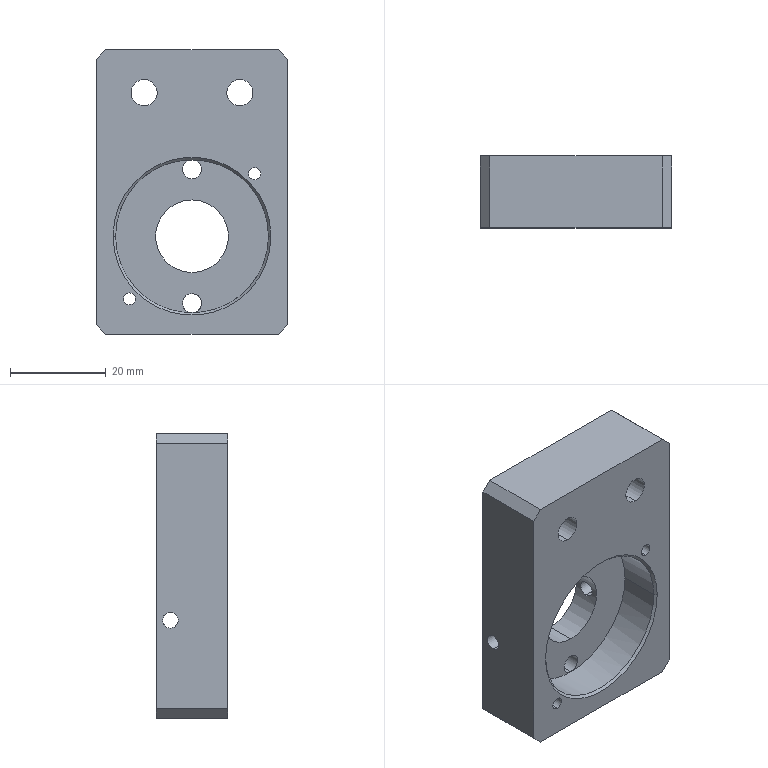Part | STEP file | Drive Shaft Bearing Housing | 1 solid | 39 faces | box 40 x 15 x 59.5 mm | volume 24876 mm3 | cylinder 24 | plane 13 | cone 2 | commonest cylinder face diameters 2.5 x4 3.3 x4 4 x4 5.5 x4 11 x4 15.2 x2